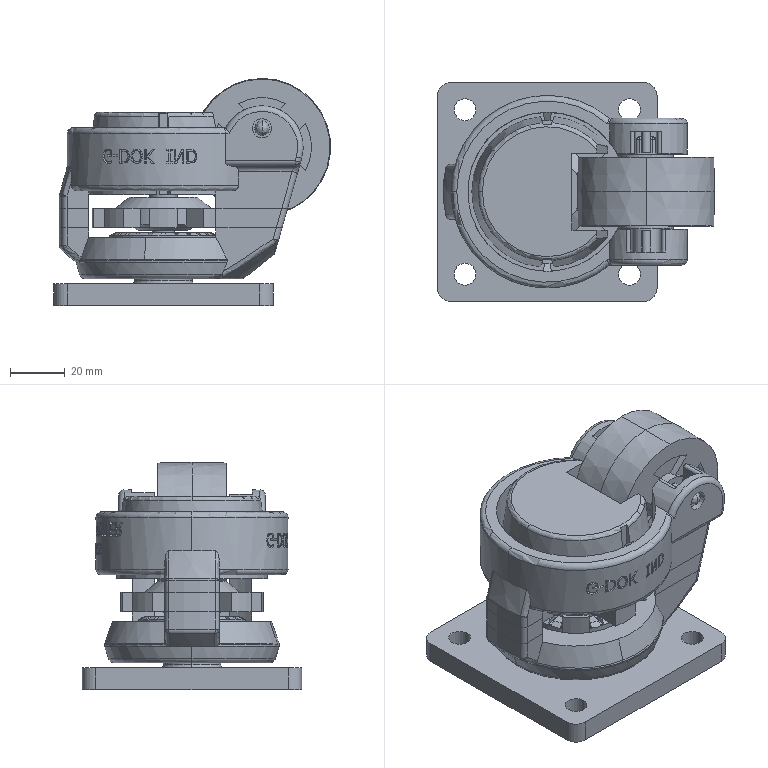Part | SolidWorks | 9 solids | 1027 faces | box 101 x 80 x 82.8 mm | volume 248675 mm3 | plane 437 | spline 224 | cylinder 219 | cone 79 | torus 44 | sphere 24 | commonest cylinder face diameters 2 x26 4 x24 68 x24 35 x16 10 x12 70 x12